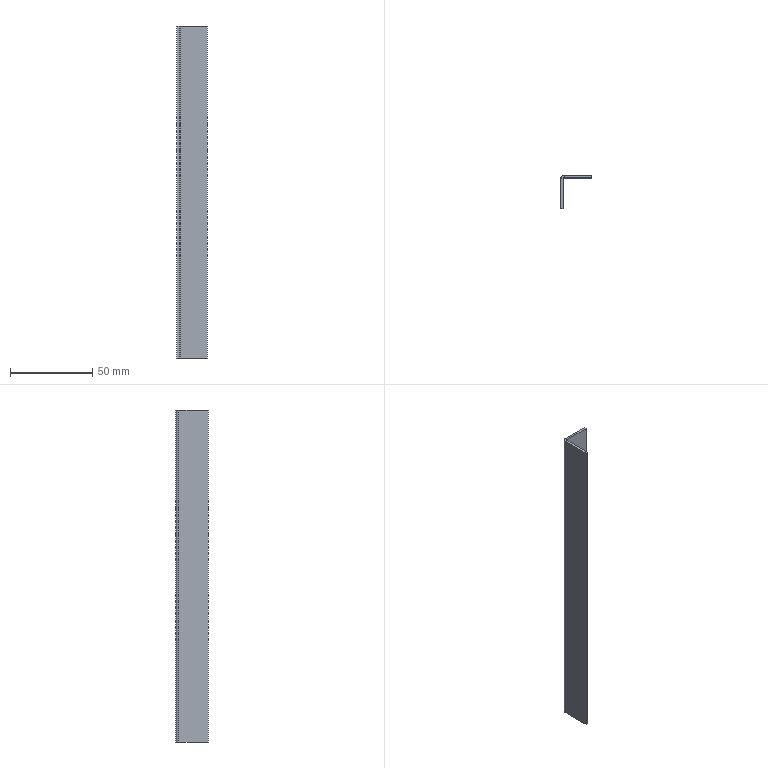Part | SolidWorks | features FlatPattern 1, SMBaseFlange 1, SheetMetal 1 | 1 solid | 14 faces | box 18.5 x 20 x 201.5 mm | volume 11021 mm3 | plane 12 | cylinder 2 | commonest cylinder face diameters 1 x1 4 x1
STEP:
#1=CARTESIAN_POINT('',(-7.504,17.789,201.5));
#2=VERTEX_POINT('',#1);
#3=CARTESIAN_POINT('',(-7.504,16.289,201.5));
#4=VERTEX_POINT('',#3);
#5=CARTESIAN_POINT('',(-7.504,17.789,201.5));
#6=DIRECTION('',(0.,-1.,0.));
#7=VECTOR('',#6,1000.);
#8=LINE('',#5,#7);
#9=EDGE_CURVE('',#2,#4,#8,.T.);
#10=ORIENTED_EDGE('',*,*,#9,.F.);
#11=CARTESIAN_POINT('',(-9.504,15.789,201.5));
#12=VERTEX_POINT('',#11);
#13=CARTESIAN_POINT('',(-7.504,15.789,201.5));
#14=DIRECTION('',(0.,0.,1.));
#15=DIRECTION('',(-1.,0.,0.));
#16=AXIS2_PLACEMENT_3D('',#13,#14,#15);
#17=CIRCLE('',#16,2.);
#18=EDGE_CURVE('',#2,#12,#17,.T.);
#19=ORIENTED_EDGE('',*,*,#18,.T.);
#20=CARTESIAN_POINT('',(-8.004,15.789,201.5));
#21=VERTEX_POINT('',#20);
#22=CARTESIAN_POINT('',(-8.004,15.789,201.5));
#23=DIRECTION('',(-1.,0.,0.));
#24=VECTOR('',#23,1000.);
#25=LINE('',#22,#24);
#26=EDGE_CURVE('',#21,#12,#25,.T.);
#27=ORIENTED_EDGE('',*,*,#26,.F.);
#28=CARTESIAN_POINT('',(-7.504,15.789,201.5));
#29=DIRECTION('',(0.,0.,1.));
#30=DIRECTION('',(1.,0.,0.));
#31=AXIS2_PLACEMENT_3D('',#28,#29,#30);
#32=CIRCLE('',#31,0.5);
#33=EDGE_CURVE('',#4,#21,#32,.T.);
#34=ORIENTED_EDGE('',*,*,#33,.F.);
#35=EDGE_LOOP('',(#10,#19,#27,#34));
#36=FACE_OUTER_BOUND('',#35,.T.);
#37=CARTESIAN_POINT('',(-7.504,17.789,201.5));
#38=DIRECTION('',(0.,0.,1.));
#39=DIRECTION('',(1.,0.,0.));
#40=AXIS2_PLACEMENT_3D('',#37,#38,#39);
#41=PLANE('',#40);
#42=ADVANCED_FACE('',(#36),#41,.T.);
#43=CARTESIAN_POINT('',(8.996,17.789,201.5));
#44=VERTEX_POINT('',#43);
#45=CARTESIAN_POINT('',(8.996,17.789,201.5));
#46=DIRECTION('',(-1.,0.,0.));
#47=VECTOR('',#46,1000.);
#48=LINE('',#45,#47);
#49=EDGE_CURVE('',#44,#2,#48,.T.);
#50=ORIENTED_EDGE('',*,*,#49,.T.);
#51=ORIENTED_EDGE('',*,*,#9,.T.);
#52=CARTESIAN_POINT('',(8.996,16.289,201.5));
#53=VERTEX_POINT('',#52);
#54=CARTESIAN_POINT('',(8.996,16.289,201.5));
#55=DIRECTION('',(-1.,0.,0.));
#56=VECTOR('',#55,1000.);
#57=LINE('',#54,#56);
#58=EDGE_CURVE('',#53,#4,#57,.T.);
#59=ORIENTED_EDGE('',*,*,#58,.F.);
#60=CARTESIAN_POINT('',(8.996,17.789,201.5));
#61=DIRECTION('',(0.,-1.,0.));
#62=VECTOR('',#61,1000.);
#63=LINE('',#60,#62);
#64=EDGE_CURVE('',#44,#53,#63,.T.);
#65=ORIENTED_EDGE('',*,*,#64,.F.);
#66=EDGE_LOOP('',(#50,#51,#59,#65));
#67=FACE_OUTER_BOUND('',#66,.T.);
#68=CARTESIAN_POINT('',(-8.004,15.789,201.5));
#69=DIRECTION('',(0.,0.,1.));
#70=DIRECTION('',(1.,0.,0.));
#71=AXIS2_PLACEMENT_3D('',#68,#69,#70);
#72=PLANE('',#71);
#73=ADVANCED_FACE('',(#67),#72,.T.);
#74=CARTESIAN_POINT('',(-9.504,15.789,0.));
#75=VERTEX_POINT('',#74);
#76=CARTESIAN_POINT('',(-8.004,15.789,0.));
#77=VERTEX_POINT('',#76);
#78=CARTESIAN_POINT('',(-9.504,15.789,0.));
#79=DIRECTION('',(1.,0.,0.));
#80=VECTOR('',#79,1000.);
#81=LINE('',#78,#80);
#82=EDGE_CURVE('',#75,#77,#81,.T.);
#83=ORIENTED_EDGE('',*,*,#82,.F.);
#84=CARTESIAN_POINT('',(-7.504,17.789,0.));
#85=VERTEX_POINT('',#84);
#86=CARTESIAN_POINT('',(-7.504,15.789,0.));
#87=DIRECTION('',(0.,0.,1.));
#88=DIRECTION('',(-1.,0.,0.));
#89=AXIS2_PLACEMENT_3D('',#86,#87,#88);
#90=CIRCLE('',#89,2.);
#91=EDGE_CURVE('',#85,#75,#90,.T.);
#92=ORIENTED_EDGE('',*,*,#91,.F.);
#93=CARTESIAN_POINT('',(-7.504,16.289,0.));
#94=VERTEX_POINT('',#93);
#95=CARTESIAN_POINT('',(-7.504,16.289,0.));
#96=DIRECTION('',(0.,1.,0.));
#97=VECTOR('',#96,1000.);
#98=LINE('',#95,#97);
#99=EDGE_CURVE('',#94,#85,#98,.T.);
#100=ORIENTED_EDGE('',*,*,#99,.F.);
#101=CARTESIAN_POINT('',(-7.504,15.789,0.));
#102=DIRECTION('',(0.,0.,1.));
#103=DIRECTION('',(1.,0.,0.));
#104=AXIS2_PLACEMENT_3D('',#101,#102,#103);
#105=CIRCLE('',#104,0.5);
#106=EDGE_CURVE('',#94,#77,#105,.T.);
#107=ORIENTED_EDGE('',*,*,#106,.T.);
#108=EDGE_LOOP('',(#83,#92,#100,#107));
#109=FACE_OUTER_BOUND('',#108,.T.);
#110=CARTESIAN_POINT('',(-9.504,15.789,0.));
#111=DIRECTION('',(0.,0.,-1.));
#112=DIRECTION('',(-1.,0.,0.));
#113=AXIS2_PLACEMENT_3D('',#110,#111,#112);
#114=PLANE('',#113);
#115=ADVANCED_FACE('',(#109),#114,.T.);
#116=CARTESIAN_POINT('',(-9.504,-2.211,0.));
#117=VERTEX_POINT('',#116);
#118=CARTESIAN_POINT('',(-9.504,17.789,0.));
#119=DIRECTION('',(0.,-1.,0.));
#120=VECTOR('',#119,1000.);
#121=LINE('',#118,#120);
#122=EDGE_CURVE('',#75,#117,#121,.T.);
#123=ORIENTED_EDGE('',*,*,#122,.F.);
#124=ORIENTED_EDGE('',*,*,#82,.T.);
#125=CARTESIAN_POINT('',(-8.004,-2.211,0.));
#126=VERTEX_POINT('',#125);
#127=CARTESIAN_POINT('',(-8.004,17.789,0.));
#128=DIRECTION('',(0.,-1.,0.));
#129=VECTOR('',#128,1000.);
#130=LINE('',#127,#129);
#131=EDGE_CURVE('',#77,#126,#130,.T.);
#132=ORIENTED_EDGE('',*,*,#131,.T.);
#133=CARTESIAN_POINT('',(-8.004,-2.211,0.));
#134=DIRECTION('',(-1.,0.,0.));
#135=VECTOR('',#134,1000.);
#136=LINE('',#133,#135);
#137=EDGE_CURVE('',#126,#117,#136,.T.);
#138=ORIENTED_EDGE('',*,*,#137,.T.);
#139=EDGE_LOOP('',(#123,#124,#132,#138));
#140=FACE_OUTER_BOUND('',#139,.T.);
#141=CARTESIAN_POINT('',(-7.504,16.289,0.));
#142=DIRECTION('',(0.,0.,-1.));
#143=DIRECTION('',(-1.,0.,0.));
#144=AXIS2_PLACEMENT_3D('',#141,#142,#143);
#145=PLANE('',#144);
#146=ADVANCED_FACE('',(#140),#145,.T.);
#147=ORIENTED_EDGE('',*,*,#122,.T.);
#148=CARTESIAN_POINT('',(-9.504,-2.211,201.5));
#149=VERTEX_POINT('',#148);
#150=CARTESIAN_POINT('',(-9.504,-2.211,201.5));
#151=DIRECTION('',(0.,0.,-1.));
#152=VECTOR('',#151,1000.);
#153=LINE('',#150,#152);
#154=EDGE_CURVE('',#149,#117,#153,.T.);
#155=ORIENTED_EDGE('',*,*,#154,.F.);
#156=CARTESIAN_POINT('',(-9.504,17.789,201.5));
#157=DIRECTION('',(0.,-1.,0.));
#158=VECTOR('',#157,1000.);
#159=LINE('',#156,#158);
#160=EDGE_CURVE('',#12,#149,#159,.T.);
#161=ORIENTED_EDGE('',*,*,#160,.F.);
#162=CARTESIAN_POINT('',(-9.504,15.789,201.5));
#163=DIRECTION('',(0.,0.,-1.));
#164=VECTOR('',#163,1000.);
#165=LINE('',#162,#164);
#166=EDGE_CURVE('',#12,#75,#165,.T.);
#167=ORIENTED_EDGE('',*,*,#166,.T.);
#168=EDGE_LOOP('',(#147,#155,#161,#167));
#169=FACE_OUTER_BOUND('',#168,.T.);
#170=CARTESIAN_POINT('',(-9.504,17.789,201.5));
#171=DIRECTION('',(1.,0.,0.));
#172=DIRECTION('',(0.,1.,0.));
#173=AXIS2_PLACEMENT_3D('',#170,#171,#172);
#174=PLANE('',#173);
#175=ADVANCED_FACE('',(#169),#174,.F.);
#176=ORIENTED_EDGE('',*,*,#137,.F.);
#177=CARTESIAN_POINT('',(-8.004,-2.211,201.5));
#178=VERTEX_POINT('',#177);
#179=CARTESIAN_POINT('',(-8.004,-2.211,201.5));
#180=DIRECTION('',(0.,0.,-1.));
#181=VECTOR('',#180,1000.);
#182=LINE('',#179,#181);
#183=EDGE_CURVE('',#178,#126,#182,.T.);
#184=ORIENTED_EDGE('',*,*,#183,.F.);
#185=CARTESIAN_POINT('',(-8.004,-2.211,201.5));
#186=DIRECTION('',(-1.,0.,0.));
#187=VECTOR('',#186,1000.);
#188=LINE('',#185,#187);
#189=EDGE_CURVE('',#178,#149,#188,.T.);
#190=ORIENTED_EDGE('',*,*,#189,.T.);
#191=ORIENTED_EDGE('',*,*,#154,.T.);
#192=EDGE_LOOP('',(#176,#184,#190,#191));
#193=FACE_OUTER_BOUND('',#192,.T.);
#194=CARTESIAN_POINT('',(-8.004,-2.211,201.5));
#195=DIRECTION('',(0.,-1.,0.));
#196=DIRECTION('',(0.,0.,-1.));
#197=AXIS2_PLACEMENT_3D('',#194,#195,#196);
#198=PLANE('',#197);
#199=ADVANCED_FACE('',(#193),#198,.T.);
#200=ORIENTED_EDGE('',*,*,#131,.F.);
#201=CARTESIAN_POINT('',(-8.004,15.789,201.5));
#202=DIRECTION('',(0.,0.,-1.));
#203=VECTOR('',#202,1000.);
#204=LINE('',#201,#203);
#205=EDGE_CURVE('',#21,#77,#204,.T.);
#206=ORIENTED_EDGE('',*,*,#205,.F.);
#207=CARTESIAN_POINT('',(-8.004,17.789,201.5));
#208=DIRECTION('',(0.,-1.,0.));
#209=VECTOR('',#208,1000.);
#210=LINE('',#207,#209);
#211=EDGE_CURVE('',#21,#178,#210,.T.);
#212=ORIENTED_EDGE('',*,*,#211,.T.);
#213=ORIENTED_EDGE('',*,*,#183,.T.);
#214=EDGE_LOOP('',(#200,#206,#212,#213));
#215=FACE_OUTER_BOUND('',#214,.T.);
#216=CARTESIAN_POINT('',(-8.004,17.789,201.5));
#217=DIRECTION('',(1.,0.,0.));
#218=DIRECTION('',(0.,1.,0.));
#219=AXIS2_PLACEMENT_3D('',#216,#217,#218);
#220=PLANE('',#219);
#221=ADVANCED_FACE('',(#215),#220,.T.);
#222=ORIENTED_EDGE('',*,*,#106,.F.);
#223=CARTESIAN_POINT('',(-7.504,16.289,201.5));
#224=DIRECTION('',(0.,0.,-1.));
#225=VECTOR('',#224,1000.);
#226=LINE('',#223,#225);
#227=EDGE_CURVE('',#4,#94,#226,.T.);
#228=ORIENTED_EDGE('',*,*,#227,.F.);
#229=ORIENTED_EDGE('',*,*,#33,.T.);
#230=ORIENTED_EDGE('',*,*,#205,.T.);
#231=EDGE_LOOP('',(#222,#228,#229,#230));
#232=FACE_OUTER_BOUND('',#231,.T.);
#233=CARTESIAN_POINT('',(-7.504,15.789,201.5));
#234=DIRECTION('',(0.,0.,-1.));
#235=DIRECTION('',(-1.,0.,0.));
#236=AXIS2_PLACEMENT_3D('',#233,#234,#235);
#237=CYLINDRICAL_SURFACE('',#236,0.5);
#238=ADVANCED_FACE('',(#232),#237,.F.);
#239=CARTESIAN_POINT('',(8.996,16.289,0.));
#240=VERTEX_POINT('',#239);
#241=CARTESIAN_POINT('',(8.996,16.289,0.));
#242=DIRECTION('',(-1.,0.,0.));
#243=VECTOR('',#242,1000.);
#244=LINE('',#241,#243);
#245=EDGE_CURVE('',#240,#94,#244,.T.);
#246=ORIENTED_EDGE('',*,*,#245,.F.);
#247=CARTESIAN_POINT('',(8.996,16.289,201.5));
#248=DIRECTION('',(0.,0.,-1.));
#249=VECTOR('',#248,1000.);
#250=LINE('',#247,#249);
#251=EDGE_CURVE('',#53,#240,#250,.T.);
#252=ORIENTED_EDGE('',*,*,#251,.F.);
#253=ORIENTED_EDGE('',*,*,#58,.T.);
#254=ORIENTED_EDGE('',*,*,#227,.T.);
#255=EDGE_LOOP('',(#246,#252,#253,#254));
#256=FACE_OUTER_BOUND('',#255,.T.);
#257=CARTESIAN_POINT('',(8.996,16.289,201.5));
#258=DIRECTION('',(0.,-1.,0.));
#259=DIRECTION('',(0.,0.,-1.));
#260=AXIS2_PLACEMENT_3D('',#257,#258,#259);
#261=PLANE('',#260);
#262=ADVANCED_FACE('',(#256),#261,.T.);
#263=CARTESIAN_POINT('',(8.996,17.789,0.));
#264=VERTEX_POINT('',#263);
#265=CARTESIAN_POINT('',(8.996,17.789,0.));
#266=DIRECTION('',(0.,-1.,0.));
#267=VECTOR('',#266,1000.);
#268=LINE('',#265,#267);
#269=EDGE_CURVE('',#264,#240,#268,.T.);
#270=ORIENTED_EDGE('',*,*,#269,.F.);
#271=CARTESIAN_POINT('',(8.996,17.789,201.5));
#272=DIRECTION('',(0.,0.,-1.));
#273=VECTOR('',#272,1000.);
#274=LINE('',#271,#273);
#275=EDGE_CURVE('',#44,#264,#274,.T.);
#276=ORIENTED_EDGE('',*,*,#275,.F.);
#277=ORIENTED_EDGE('',*,*,#64,.T.);
#278=ORIENTED_EDGE('',*,*,#251,.T.);
#279=EDGE_LOOP('',(#270,#276,#277,#278));
#280=FACE_OUTER_BOUND('',#279,.T.);
#281=CARTESIAN_POINT('',(8.996,17.789,201.5));
#282=DIRECTION('',(1.,0.,0.));
#283=DIRECTION('',(0.,0.,-1.));
#284=AXIS2_PLACEMENT_3D('',#281,#282,#283);
#285=PLANE('',#284);
#286=ADVANCED_FACE('',(#280),#285,.T.);
#287=CARTESIAN_POINT('',(8.996,17.789,0.));
#288=DIRECTION('',(-1.,0.,0.));
#289=VECTOR('',#288,1000.);
#290=LINE('',#287,#289);
#291=EDGE_CURVE('',#264,#85,#290,.T.);
#292=ORIENTED_EDGE('',*,*,#291,.T.);
#293=CARTESIAN_POINT('',(-7.504,17.789,201.5));
#294=DIRECTION('',(0.,0.,-1.));
#295=VECTOR('',#294,1000.);
#296=LINE('',#293,#295);
#297=EDGE_CURVE('',#2,#85,#296,.T.);
#298=ORIENTED_EDGE('',*,*,#297,.F.);
#299=ORIENTED_EDGE('',*,*,#49,.F.);
#300=ORIENTED_EDGE('',*,*,#275,.T.);
#301=EDGE_LOOP('',(#292,#298,#299,#300));
#302=FACE_OUTER_BOUND('',#301,.T.);
#303=CARTESIAN_POINT('',(8.996,17.789,201.5));
#304=DIRECTION('',(0.,-1.,0.));
#305=DIRECTION('',(0.,0.,-1.));
#306=AXIS2_PLACEMENT_3D('',#303,#304,#305);
#307=PLANE('',#306);
#308=ADVANCED_FACE('',(#302),#307,.F.);
#309=ORIENTED_EDGE('',*,*,#91,.T.);
#310=ORIENTED_EDGE('',*,*,#166,.F.);
#311=ORIENTED_EDGE('',*,*,#18,.F.);
#312=ORIENTED_EDGE('',*,*,#297,.T.);
#313=EDGE_LOOP('',(#309,#310,#311,#312));
#314=FACE_OUTER_BOUND('',#313,.T.);
#315=CARTESIAN_POINT('',(-7.504,15.789,201.5));
#316=DIRECTION('',(0.,0.,-1.));
#317=DIRECTION('',(-1.,0.,0.));
#318=AXIS2_PLACEMENT_3D('',#315,#316,#317);
#319=CYLINDRICAL_SURFACE('',#318,2.);
#320=ADVANCED_FACE('',(#314),#319,.T.);
#321=ORIENTED_EDGE('',*,*,#160,.T.);
#322=ORIENTED_EDGE('',*,*,#189,.F.);
#323=ORIENTED_EDGE('',*,*,#211,.F.);
#324=ORIENTED_EDGE('',*,*,#26,.T.);
#325=EDGE_LOOP('',(#321,#322,#323,#324));
#326=FACE_OUTER_BOUND('',#325,.T.);
#327=CARTESIAN_POINT('',(-7.504,15.789,201.5));
#328=DIRECTION('',(0.,0.,1.));
#329=DIRECTION('',(1.,0.,0.));
#330=AXIS2_PLACEMENT_3D('',#327,#328,#329);
#331=PLANE('',#330);
#332=ADVANCED_FACE('',(#326),#331,.T.);
#333=ORIENTED_EDGE('',*,*,#245,.T.);
#334=ORIENTED_EDGE('',*,*,#99,.T.);
#335=ORIENTED_EDGE('',*,*,#291,.F.);
#336=ORIENTED_EDGE('',*,*,#269,.T.);
#337=EDGE_LOOP('',(#333,#334,#335,#336));
#338=FACE_OUTER_BOUND('',#337,.T.);
#339=CARTESIAN_POINT('',(-7.504,15.789,0.));
#340=DIRECTION('',(0.,0.,1.));
#341=DIRECTION('',(1.,0.,0.));
#342=AXIS2_PLACEMENT_3D('',#339,#340,#341);
#343=PLANE('',#342);
#344=ADVANCED_FACE('',(#338),#343,.F.);
#345=CLOSED_SHELL('',(#42,#73,#115,#146,#175,#199,#221,#238,#262,#286,#308,#320,#332,#344));
#346=MANIFOLD_SOLID_BREP('',#345);
#347=CARTESIAN_POINT('',(0.,0.,0.));
#348=DIRECTION('',(0.,0.,1.));
#349=DIRECTION('',(1.,0.,0.));
#350=AXIS2_PLACEMENT_3D('',#347,#348,#349);
#351=(LENGTH_UNIT()NAMED_UNIT(*)SI_UNIT(.MILLI.,.METRE.));
#352=UNCERTAINTY_MEASURE_WITH_UNIT(LENGTH_MEASURE(0.00001),#351,'','');
#353=(NAMED_UNIT(*)PLANE_ANGLE_UNIT()SI_UNIT($,.RADIAN.));
#354=(NAMED_UNIT(*)SI_UNIT($,.STERADIAN.)SOLID_ANGLE_UNIT());
#355=(GEOMETRIC_REPRESENTATION_CONTEXT(3)GLOBAL_UNCERTAINTY_ASSIGNED_CONTEXT((#352))GLOBAL_UNIT_ASSIGNED_CONTEXT((#351,#353,#354))REPRESENTATION_CONTEXT('',''));
#356=ADVANCED_BREP_SHAPE_REPRESENTATION('',(#346,#350),#355);